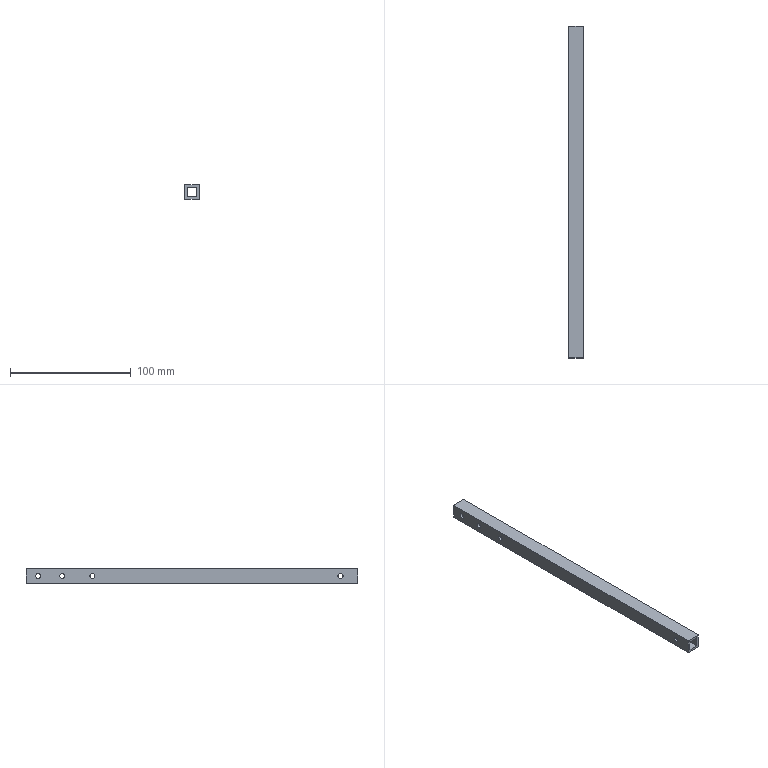Part | SolidWorks | features ICE 3, Extrusion 1 | 1 solid | 26 faces | box 12 x 275 x 12 mm | volume 21786 mm3 | cylinder 16 | plane 10 | commonest cylinder face diameters 4.1 x12 4.2 x4
STEP:
#1=CARTESIAN_POINT('',(6.,265.,-2.05));
#2=VERTEX_POINT('',#1);
#3=CARTESIAN_POINT('',(6.,265.,2.05));
#4=VERTEX_POINT('',#3);
#5=CARTESIAN_POINT('',(6.,265.,0.));
#6=DIRECTION('',(-1.,0.,0.));
#7=DIRECTION('',(0.,0.,1.));
#8=AXIS2_PLACEMENT_3D('',#5,#6,#7);
#9=CIRCLE('',#8,2.05);
#10=EDGE_CURVE('',#2,#4,#9,.T.);
#11=ORIENTED_EDGE('',*,*,#10,.F.);
#12=CARTESIAN_POINT('',(4.,265.,-2.05));
#13=VERTEX_POINT('',#12);
#14=CARTESIAN_POINT('',(6.,265.,-2.05));
#15=DIRECTION('',(-1.,0.,0.));
#16=VECTOR('',#15,1000.);
#17=LINE('',#14,#16);
#18=EDGE_CURVE('',#2,#13,#17,.T.);
#19=ORIENTED_EDGE('',*,*,#18,.T.);
#20=CARTESIAN_POINT('',(4.,265.,2.05));
#21=VERTEX_POINT('',#20);
#22=CARTESIAN_POINT('',(4.,265.,0.));
#23=DIRECTION('',(-1.,0.,0.));
#24=DIRECTION('',(0.,0.,1.));
#25=AXIS2_PLACEMENT_3D('',#22,#23,#24);
#26=CIRCLE('',#25,2.05);
#27=EDGE_CURVE('',#13,#21,#26,.T.);
#28=ORIENTED_EDGE('',*,*,#27,.T.);
#29=CARTESIAN_POINT('',(6.,265.,2.05));
#30=DIRECTION('',(-1.,0.,0.));
#31=VECTOR('',#30,1000.);
#32=LINE('',#29,#31);
#33=EDGE_CURVE('',#4,#21,#32,.T.);
#34=ORIENTED_EDGE('',*,*,#33,.F.);
#35=EDGE_LOOP('',(#11,#19,#28,#34));
#36=FACE_OUTER_BOUND('',#35,.T.);
#37=CARTESIAN_POINT('',(6.,265.,0.));
#38=DIRECTION('',(-1.,0.,0.));
#39=DIRECTION('',(0.,0.,1.));
#40=AXIS2_PLACEMENT_3D('',#37,#38,#39);
#41=CYLINDRICAL_SURFACE('',#40,2.05);
#42=ADVANCED_FACE('',(#36),#41,.F.);
#43=CARTESIAN_POINT('',(6.,245.,-2.05));
#44=VERTEX_POINT('',#43);
#45=CARTESIAN_POINT('',(6.,245.,2.05));
#46=VERTEX_POINT('',#45);
#47=CARTESIAN_POINT('',(6.,245.,0.));
#48=DIRECTION('',(-1.,0.,0.));
#49=DIRECTION('',(0.,0.,1.));
#50=AXIS2_PLACEMENT_3D('',#47,#48,#49);
#51=CIRCLE('',#50,2.05);
#52=EDGE_CURVE('',#44,#46,#51,.T.);
#53=ORIENTED_EDGE('',*,*,#52,.F.);
#54=CARTESIAN_POINT('',(4.,245.,-2.05));
#55=VERTEX_POINT('',#54);
#56=CARTESIAN_POINT('',(6.,245.,-2.05));
#57=DIRECTION('',(-1.,0.,0.));
#58=VECTOR('',#57,1000.);
#59=LINE('',#56,#58);
#60=EDGE_CURVE('',#44,#55,#59,.T.);
#61=ORIENTED_EDGE('',*,*,#60,.T.);
#62=CARTESIAN_POINT('',(4.,245.,2.05));
#63=VERTEX_POINT('',#62);
#64=CARTESIAN_POINT('',(4.,245.,0.));
#65=DIRECTION('',(-1.,0.,0.));
#66=DIRECTION('',(0.,0.,1.));
#67=AXIS2_PLACEMENT_3D('',#64,#65,#66);
#68=CIRCLE('',#67,2.05);
#69=EDGE_CURVE('',#55,#63,#68,.T.);
#70=ORIENTED_EDGE('',*,*,#69,.T.);
#71=CARTESIAN_POINT('',(6.,245.,2.05));
#72=DIRECTION('',(-1.,0.,0.));
#73=VECTOR('',#72,1000.);
#74=LINE('',#71,#73);
#75=EDGE_CURVE('',#46,#63,#74,.T.);
#76=ORIENTED_EDGE('',*,*,#75,.F.);
#77=EDGE_LOOP('',(#53,#61,#70,#76));
#78=FACE_OUTER_BOUND('',#77,.T.);
#79=CARTESIAN_POINT('',(6.,245.,0.));
#80=DIRECTION('',(-1.,0.,0.));
#81=DIRECTION('',(0.,0.,1.));
#82=AXIS2_PLACEMENT_3D('',#79,#80,#81);
#83=CYLINDRICAL_SURFACE('',#82,2.05);
#84=ADVANCED_FACE('',(#78),#83,.F.);
#85=CARTESIAN_POINT('',(6.,220.,-2.05));
#86=VERTEX_POINT('',#85);
#87=CARTESIAN_POINT('',(6.,220.,2.05));
#88=VERTEX_POINT('',#87);
#89=CARTESIAN_POINT('',(6.,220.,0.));
#90=DIRECTION('',(-1.,0.,0.));
#91=DIRECTION('',(0.,0.,1.));
#92=AXIS2_PLACEMENT_3D('',#89,#90,#91);
#93=CIRCLE('',#92,2.05);
#94=EDGE_CURVE('',#86,#88,#93,.T.);
#95=ORIENTED_EDGE('',*,*,#94,.F.);
#96=CARTESIAN_POINT('',(4.,220.,-2.05));
#97=VERTEX_POINT('',#96);
#98=CARTESIAN_POINT('',(6.,220.,-2.05));
#99=DIRECTION('',(-1.,0.,0.));
#100=VECTOR('',#99,1000.);
#101=LINE('',#98,#100);
#102=EDGE_CURVE('',#86,#97,#101,.T.);
#103=ORIENTED_EDGE('',*,*,#102,.T.);
#104=CARTESIAN_POINT('',(4.,220.,2.05));
#105=VERTEX_POINT('',#104);
#106=CARTESIAN_POINT('',(4.,220.,0.));
#107=DIRECTION('',(-1.,0.,0.));
#108=DIRECTION('',(0.,0.,1.));
#109=AXIS2_PLACEMENT_3D('',#106,#107,#108);
#110=CIRCLE('',#109,2.05);
#111=EDGE_CURVE('',#97,#105,#110,.T.);
#112=ORIENTED_EDGE('',*,*,#111,.T.);
#113=CARTESIAN_POINT('',(6.,220.,2.05));
#114=DIRECTION('',(-1.,0.,0.));
#115=VECTOR('',#114,1000.);
#116=LINE('',#113,#115);
#117=EDGE_CURVE('',#88,#105,#116,.T.);
#118=ORIENTED_EDGE('',*,*,#117,.F.);
#119=EDGE_LOOP('',(#95,#103,#112,#118));
#120=FACE_OUTER_BOUND('',#119,.T.);
#121=CARTESIAN_POINT('',(6.,220.,0.));
#122=DIRECTION('',(-1.,0.,0.));
#123=DIRECTION('',(0.,0.,1.));
#124=AXIS2_PLACEMENT_3D('',#121,#122,#123);
#125=CYLINDRICAL_SURFACE('',#124,2.05);
#126=ADVANCED_FACE('',(#120),#125,.F.);
#127=CARTESIAN_POINT('',(6.,14.5,-2.1));
#128=VERTEX_POINT('',#127);
#129=CARTESIAN_POINT('',(6.,14.5,2.1));
#130=VERTEX_POINT('',#129);
#131=CARTESIAN_POINT('',(6.,14.5,0.));
#132=DIRECTION('',(-1.,0.,0.));
#133=DIRECTION('',(0.,0.,1.));
#134=AXIS2_PLACEMENT_3D('',#131,#132,#133);
#135=CIRCLE('',#134,2.1);
#136=EDGE_CURVE('',#128,#130,#135,.T.);
#137=ORIENTED_EDGE('',*,*,#136,.F.);
#138=CARTESIAN_POINT('',(4.,14.5,-2.1));
#139=VERTEX_POINT('',#138);
#140=CARTESIAN_POINT('',(6.,14.5,-2.1));
#141=DIRECTION('',(-1.,0.,0.));
#142=VECTOR('',#141,1000.);
#143=LINE('',#140,#142);
#144=EDGE_CURVE('',#128,#139,#143,.T.);
#145=ORIENTED_EDGE('',*,*,#144,.T.);
#146=CARTESIAN_POINT('',(4.,14.5,2.1));
#147=VERTEX_POINT('',#146);
#148=CARTESIAN_POINT('',(4.,14.5,0.));
#149=DIRECTION('',(-1.,0.,0.));
#150=DIRECTION('',(0.,0.,1.));
#151=AXIS2_PLACEMENT_3D('',#148,#149,#150);
#152=CIRCLE('',#151,2.1);
#153=EDGE_CURVE('',#139,#147,#152,.T.);
#154=ORIENTED_EDGE('',*,*,#153,.T.);
#155=CARTESIAN_POINT('',(6.,14.5,2.1));
#156=DIRECTION('',(-1.,0.,0.));
#157=VECTOR('',#156,1000.);
#158=LINE('',#155,#157);
#159=EDGE_CURVE('',#130,#147,#158,.T.);
#160=ORIENTED_EDGE('',*,*,#159,.F.);
#161=EDGE_LOOP('',(#137,#145,#154,#160));
#162=FACE_OUTER_BOUND('',#161,.T.);
#163=CARTESIAN_POINT('',(6.,14.5,0.));
#164=DIRECTION('',(-1.,0.,0.));
#165=DIRECTION('',(0.,0.,1.));
#166=AXIS2_PLACEMENT_3D('',#163,#164,#165);
#167=CYLINDRICAL_SURFACE('',#166,2.1);
#168=ADVANCED_FACE('',(#162),#167,.F.);
#169=CARTESIAN_POINT('',(-4.,265.,2.05));
#170=VERTEX_POINT('',#169);
#171=CARTESIAN_POINT('',(-4.,265.,-2.05));
#172=VERTEX_POINT('',#171);
#173=CARTESIAN_POINT('',(-4.,265.,0.));
#174=DIRECTION('',(1.,0.,0.));
#175=DIRECTION('',(0.,0.,-1.));
#176=AXIS2_PLACEMENT_3D('',#173,#174,#175);
#177=CIRCLE('',#176,2.05);
#178=EDGE_CURVE('',#170,#172,#177,.T.);
#179=ORIENTED_EDGE('',*,*,#178,.T.);
#180=CARTESIAN_POINT('',(-6.,265.,-2.05));
#181=VERTEX_POINT('',#180);
#182=CARTESIAN_POINT('',(6.,265.,-2.05));
#183=DIRECTION('',(-1.,0.,0.));
#184=VECTOR('',#183,1000.);
#185=LINE('',#182,#184);
#186=EDGE_CURVE('',#172,#181,#185,.T.);
#187=ORIENTED_EDGE('',*,*,#186,.T.);
#188=CARTESIAN_POINT('',(-6.,265.,2.05));
#189=VERTEX_POINT('',#188);
#190=CARTESIAN_POINT('',(-6.,265.,0.));
#191=DIRECTION('',(-1.,0.,0.));
#192=DIRECTION('',(0.,0.,1.));
#193=AXIS2_PLACEMENT_3D('',#190,#191,#192);
#194=CIRCLE('',#193,2.05);
#195=EDGE_CURVE('',#181,#189,#194,.T.);
#196=ORIENTED_EDGE('',*,*,#195,.T.);
#197=CARTESIAN_POINT('',(6.,265.,2.05));
#198=DIRECTION('',(-1.,0.,0.));
#199=VECTOR('',#198,1000.);
#200=LINE('',#197,#199);
#201=EDGE_CURVE('',#170,#189,#200,.T.);
#202=ORIENTED_EDGE('',*,*,#201,.F.);
#203=EDGE_LOOP('',(#179,#187,#196,#202));
#204=FACE_OUTER_BOUND('',#203,.T.);
#205=CARTESIAN_POINT('',(6.,265.,0.));
#206=DIRECTION('',(-1.,0.,0.));
#207=DIRECTION('',(0.,0.,1.));
#208=AXIS2_PLACEMENT_3D('',#205,#206,#207);
#209=CYLINDRICAL_SURFACE('',#208,2.05);
#210=ADVANCED_FACE('',(#204),#209,.F.);
#211=CARTESIAN_POINT('',(-4.,245.,2.05));
#212=VERTEX_POINT('',#211);
#213=CARTESIAN_POINT('',(-4.,245.,-2.05));
#214=VERTEX_POINT('',#213);
#215=CARTESIAN_POINT('',(-4.,245.,0.));
#216=DIRECTION('',(1.,0.,0.));
#217=DIRECTION('',(0.,0.,-1.));
#218=AXIS2_PLACEMENT_3D('',#215,#216,#217);
#219=CIRCLE('',#218,2.05);
#220=EDGE_CURVE('',#212,#214,#219,.T.);
#221=ORIENTED_EDGE('',*,*,#220,.T.);
#222=CARTESIAN_POINT('',(-6.,245.,-2.05));
#223=VERTEX_POINT('',#222);
#224=CARTESIAN_POINT('',(6.,245.,-2.05));
#225=DIRECTION('',(-1.,0.,0.));
#226=VECTOR('',#225,1000.);
#227=LINE('',#224,#226);
#228=EDGE_CURVE('',#214,#223,#227,.T.);
#229=ORIENTED_EDGE('',*,*,#228,.T.);
#230=CARTESIAN_POINT('',(-6.,245.,2.05));
#231=VERTEX_POINT('',#230);
#232=CARTESIAN_POINT('',(-6.,245.,0.));
#233=DIRECTION('',(-1.,0.,0.));
#234=DIRECTION('',(0.,0.,1.));
#235=AXIS2_PLACEMENT_3D('',#232,#233,#234);
#236=CIRCLE('',#235,2.05);
#237=EDGE_CURVE('',#223,#231,#236,.T.);
#238=ORIENTED_EDGE('',*,*,#237,.T.);
#239=CARTESIAN_POINT('',(6.,245.,2.05));
#240=DIRECTION('',(-1.,0.,0.));
#241=VECTOR('',#240,1000.);
#242=LINE('',#239,#241);
#243=EDGE_CURVE('',#212,#231,#242,.T.);
#244=ORIENTED_EDGE('',*,*,#243,.F.);
#245=EDGE_LOOP('',(#221,#229,#238,#244));
#246=FACE_OUTER_BOUND('',#245,.T.);
#247=CARTESIAN_POINT('',(6.,245.,0.));
#248=DIRECTION('',(-1.,0.,0.));
#249=DIRECTION('',(0.,0.,1.));
#250=AXIS2_PLACEMENT_3D('',#247,#248,#249);
#251=CYLINDRICAL_SURFACE('',#250,2.05);
#252=ADVANCED_FACE('',(#246),#251,.F.);
#253=CARTESIAN_POINT('',(-4.,220.,2.05));
#254=VERTEX_POINT('',#253);
#255=CARTESIAN_POINT('',(-4.,220.,-2.05));
#256=VERTEX_POINT('',#255);
#257=CARTESIAN_POINT('',(-4.,220.,0.));
#258=DIRECTION('',(1.,0.,0.));
#259=DIRECTION('',(0.,0.,-1.));
#260=AXIS2_PLACEMENT_3D('',#257,#258,#259);
#261=CIRCLE('',#260,2.05);
#262=EDGE_CURVE('',#254,#256,#261,.T.);
#263=ORIENTED_EDGE('',*,*,#262,.T.);
#264=CARTESIAN_POINT('',(-6.,220.,-2.05));
#265=VERTEX_POINT('',#264);
#266=CARTESIAN_POINT('',(6.,220.,-2.05));
#267=DIRECTION('',(-1.,0.,0.));
#268=VECTOR('',#267,1000.);
#269=LINE('',#266,#268);
#270=EDGE_CURVE('',#256,#265,#269,.T.);
#271=ORIENTED_EDGE('',*,*,#270,.T.);
#272=CARTESIAN_POINT('',(-6.,220.,2.05));
#273=VERTEX_POINT('',#272);
#274=CARTESIAN_POINT('',(-6.,220.,0.));
#275=DIRECTION('',(-1.,0.,0.));
#276=DIRECTION('',(0.,0.,1.));
#277=AXIS2_PLACEMENT_3D('',#274,#275,#276);
#278=CIRCLE('',#277,2.05);
#279=EDGE_CURVE('',#265,#273,#278,.T.);
#280=ORIENTED_EDGE('',*,*,#279,.T.);
#281=CARTESIAN_POINT('',(6.,220.,2.05));
#282=DIRECTION('',(-1.,0.,0.));
#283=VECTOR('',#282,1000.);
#284=LINE('',#281,#283);
#285=EDGE_CURVE('',#254,#273,#284,.T.);
#286=ORIENTED_EDGE('',*,*,#285,.F.);
#287=EDGE_LOOP('',(#263,#271,#280,#286));
#288=FACE_OUTER_BOUND('',#287,.T.);
#289=CARTESIAN_POINT('',(6.,220.,0.));
#290=DIRECTION('',(-1.,0.,0.));
#291=DIRECTION('',(0.,0.,1.));
#292=AXIS2_PLACEMENT_3D('',#289,#290,#291);
#293=CYLINDRICAL_SURFACE('',#292,2.05);
#294=ADVANCED_FACE('',(#288),#293,.F.);
#295=CARTESIAN_POINT('',(-4.,14.5,2.1));
#296=VERTEX_POINT('',#295);
#297=CARTESIAN_POINT('',(-4.,14.5,-2.1));
#298=VERTEX_POINT('',#297);
#299=CARTESIAN_POINT('',(-4.,14.5,0.));
#300=DIRECTION('',(1.,0.,0.));
#301=DIRECTION('',(0.,0.,-1.));
#302=AXIS2_PLACEMENT_3D('',#299,#300,#301);
#303=CIRCLE('',#302,2.1);
#304=EDGE_CURVE('',#296,#298,#303,.T.);
#305=ORIENTED_EDGE('',*,*,#304,.T.);
#306=CARTESIAN_POINT('',(-6.,14.5,-2.1));
#307=VERTEX_POINT('',#306);
#308=CARTESIAN_POINT('',(6.,14.5,-2.1));
#309=DIRECTION('',(-1.,0.,0.));
#310=VECTOR('',#309,1000.);
#311=LINE('',#308,#310);
#312=EDGE_CURVE('',#298,#307,#311,.T.);
#313=ORIENTED_EDGE('',*,*,#312,.T.);
#314=CARTESIAN_POINT('',(-6.,14.5,2.1));
#315=VERTEX_POINT('',#314);
#316=CARTESIAN_POINT('',(-6.,14.5,0.));
#317=DIRECTION('',(-1.,0.,0.));
#318=DIRECTION('',(0.,0.,1.));
#319=AXIS2_PLACEMENT_3D('',#316,#317,#318);
#320=CIRCLE('',#319,2.1);
#321=EDGE_CURVE('',#307,#315,#320,.T.);
#322=ORIENTED_EDGE('',*,*,#321,.T.);
#323=CARTESIAN_POINT('',(6.,14.5,2.1));
#324=DIRECTION('',(-1.,0.,0.));
#325=VECTOR('',#324,1000.);
#326=LINE('',#323,#325);
#327=EDGE_CURVE('',#296,#315,#326,.T.);
#328=ORIENTED_EDGE('',*,*,#327,.F.);
#329=EDGE_LOOP('',(#305,#313,#322,#328));
#330=FACE_OUTER_BOUND('',#329,.T.);
#331=CARTESIAN_POINT('',(6.,14.5,0.));
#332=DIRECTION('',(-1.,0.,0.));
#333=DIRECTION('',(0.,0.,1.));
#334=AXIS2_PLACEMENT_3D('',#331,#332,#333);
#335=CYLINDRICAL_SURFACE('',#334,2.1);
#336=ADVANCED_FACE('',(#330),#335,.F.);
#337=CARTESIAN_POINT('',(6.,275.,6.));
#338=VERTEX_POINT('',#337);
#339=CARTESIAN_POINT('',(6.,275.,-6.));
#340=VERTEX_POINT('',#339);
#341=CARTESIAN_POINT('',(6.,275.,-6.));
#342=DIRECTION('',(0.,0.,-1.));
#343=VECTOR('',#342,1000.);
#344=LINE('',#341,#343);
#345=EDGE_CURVE('',#338,#340,#344,.T.);
#346=ORIENTED_EDGE('',*,*,#345,.T.);
#347=CARTESIAN_POINT('',(-6.,275.,-6.));
#348=VERTEX_POINT('',#347);
#349=CARTESIAN_POINT('',(-6.,275.,-6.));
#350=DIRECTION('',(-1.,0.,0.));
#351=VECTOR('',#350,1000.);
#352=LINE('',#349,#351);
#353=EDGE_CURVE('',#340,#348,#352,.T.);
#354=ORIENTED_EDGE('',*,*,#353,.T.);
#355=CARTESIAN_POINT('',(-6.,275.,6.));
#356=VERTEX_POINT('',#355);
#357=CARTESIAN_POINT('',(-6.,275.,-6.));
#358=DIRECTION('',(0.,0.,1.));
#359=VECTOR('',#358,1000.);
#360=LINE('',#357,#359);
#361=EDGE_CURVE('',#348,#356,#360,.T.);
#362=ORIENTED_EDGE('',*,*,#361,.T.);
#363=CARTESIAN_POINT('',(-6.,275.,6.));
#364=DIRECTION('',(1.,0.,0.));
#365=VECTOR('',#364,1000.);
#366=LINE('',#363,#365);
#367=EDGE_CURVE('',#356,#338,#366,.T.);
#368=ORIENTED_EDGE('',*,*,#367,.T.);
#369=EDGE_LOOP('',(#346,#354,#362,#368));
#370=FACE_OUTER_BOUND('',#369,.T.);
#371=CARTESIAN_POINT('',(4.,275.,-4.));
#372=VERTEX_POINT('',#371);
#373=CARTESIAN_POINT('',(-4.,275.,-4.));
#374=VERTEX_POINT('',#373);
#375=CARTESIAN_POINT('',(-4.,275.,-4.));
#376=DIRECTION('',(-1.,0.,0.));
#377=VECTOR('',#376,1000.);
#378=LINE('',#375,#377);
#379=EDGE_CURVE('',#372,#374,#378,.T.);
#380=ORIENTED_EDGE('',*,*,#379,.F.);
#381=CARTESIAN_POINT('',(4.,275.,4.));
#382=VERTEX_POINT('',#381);
#383=CARTESIAN_POINT('',(4.,275.,-4.));
#384=DIRECTION('',(0.,0.,-1.));
#385=VECTOR('',#384,1000.);
#386=LINE('',#383,#385);
#387=EDGE_CURVE('',#382,#372,#386,.T.);
#388=ORIENTED_EDGE('',*,*,#387,.F.);
#389=CARTESIAN_POINT('',(-4.,275.,4.));
#390=VERTEX_POINT('',#389);
#391=CARTESIAN_POINT('',(-4.,275.,4.));
#392=DIRECTION('',(1.,0.,0.));
#393=VECTOR('',#392,1000.);
#394=LINE('',#391,#393);
#395=EDGE_CURVE('',#390,#382,#394,.T.);
#396=ORIENTED_EDGE('',*,*,#395,.F.);
#397=CARTESIAN_POINT('',(-4.,275.,-4.));
#398=DIRECTION('',(0.,0.,1.));
#399=VECTOR('',#398,1000.);
#400=LINE('',#397,#399);
#401=EDGE_CURVE('',#374,#390,#400,.T.);
#402=ORIENTED_EDGE('',*,*,#401,.F.);
#403=EDGE_LOOP('',(#380,#388,#396,#402));
#404=FACE_BOUND('',#403,.T.);
#405=CARTESIAN_POINT('',(0.,275.,0.));
#406=DIRECTION('',(0.,1.,0.));
#407=DIRECTION('',(0.,0.,1.));
#408=AXIS2_PLACEMENT_3D('',#405,#406,#407);
#409=PLANE('',#408);
#410=ADVANCED_FACE('',(#370,#404),#409,.T.);
#411=CARTESIAN_POINT('',(6.,0.,6.));
#412=VERTEX_POINT('',#411);
#413=CARTESIAN_POINT('',(6.,0.,-6.));
#414=VERTEX_POINT('',#413);
#415=CARTESIAN_POINT('',(6.,0.,-6.));
#416=DIRECTION('',(0.,0.,-1.));
#417=VECTOR('',#416,1000.);
#418=LINE('',#415,#417);
#419=EDGE_CURVE('',#412,#414,#418,.T.);
#420=ORIENTED_EDGE('',*,*,#419,.F.);
#421=CARTESIAN_POINT('',(-6.,0.,6.));
#422=VERTEX_POINT('',#421);
#423=CARTESIAN_POINT('',(-6.,0.,6.));
#424=DIRECTION('',(1.,0.,0.));
#425=VECTOR('',#424,1000.);
#426=LINE('',#423,#425);
#427=EDGE_CURVE('',#422,#412,#426,.T.);
#428=ORIENTED_EDGE('',*,*,#427,.F.);
#429=CARTESIAN_POINT('',(-6.,0.,-6.));
#430=VERTEX_POINT('',#429);
#431=CARTESIAN_POINT('',(-6.,0.,-6.));
#432=DIRECTION('',(0.,0.,1.));
#433=VECTOR('',#432,1000.);
#434=LINE('',#431,#433);
#435=EDGE_CURVE('',#430,#422,#434,.T.);
#436=ORIENTED_EDGE('',*,*,#435,.F.);
#437=CARTESIAN_POINT('',(-6.,0.,-6.));
#438=DIRECTION('',(-1.,0.,0.));
#439=VECTOR('',#438,1000.);
#440=LINE('',#437,#439);
#441=EDGE_CURVE('',#414,#430,#440,.T.);
#442=ORIENTED_EDGE('',*,*,#441,.F.);
#443=EDGE_LOOP('',(#420,#428,#436,#442));
#444=FACE_OUTER_BOUND('',#443,.T.);
#445=CARTESIAN_POINT('',(4.,0.,4.));
#446=VERTEX_POINT('',#445);
#447=CARTESIAN_POINT('',(4.,0.,-4.));
#448=VERTEX_POINT('',#447);
#449=CARTESIAN_POINT('',(4.,0.,-4.));
#450=DIRECTION('',(0.,0.,-1.));
#451=VECTOR('',#450,1000.);
#452=LINE('',#449,#451);
#453=EDGE_CURVE('',#446,#448,#452,.T.);
#454=ORIENTED_EDGE('',*,*,#453,.T.);
#455=CARTESIAN_POINT('',(-4.,0.,-4.));
#456=VERTEX_POINT('',#455);
#457=CARTESIAN_POINT('',(-4.,0.,-4.));
#458=DIRECTION('',(-1.,0.,0.));
#459=VECTOR('',#458,1000.);
#460=LINE('',#457,#459);
#461=EDGE_CURVE('',#448,#456,#460,.T.);
#462=ORIENTED_EDGE('',*,*,#461,.T.);
#463=CARTESIAN_POINT('',(-4.,0.,4.));
#464=VERTEX_POINT('',#463);
#465=CARTESIAN_POINT('',(-4.,0.,-4.));
#466=DIRECTION('',(0.,0.,1.));
#467=VECTOR('',#466,1000.);
#468=LINE('',#465,#467);
#469=EDGE_CURVE('',#456,#464,#468,.T.);
#470=ORIENTED_EDGE('',*,*,#469,.T.);
#471=CARTESIAN_POINT('',(-4.,0.,4.));
#472=DIRECTION('',(1.,0.,0.));
#473=VECTOR('',#472,1000.);
#474=LINE('',#471,#473);
#475=EDGE_CURVE('',#464,#446,#474,.T.);
#476=ORIENTED_EDGE('',*,*,#475,.T.);
#477=EDGE_LOOP('',(#454,#462,#470,#476));
#478=FACE_BOUND('',#477,.T.);
#479=CARTESIAN_POINT('',(0.,0.,0.));
#480=DIRECTION('',(0.,1.,0.));
#481=DIRECTION('',(0.,0.,1.));
#482=AXIS2_PLACEMENT_3D('',#479,#480,#481);
#483=PLANE('',#482);
#484=ADVANCED_FACE('',(#444,#478),#483,.F.);
#485=CARTESIAN_POINT('',(6.,265.,0.));
#486=DIRECTION('',(-1.,0.,0.));
#487=DIRECTION('',(0.,0.,1.));
#488=AXIS2_PLACEMENT_3D('',#485,#486,#487);
#489=CIRCLE('',#488,2.05);
#490=EDGE_CURVE('',#4,#2,#489,.T.);
#491=ORIENTED_EDGE('',*,*,#490,.T.);
#492=ORIENTED_EDGE('',*,*,#10,.T.);
#493=EDGE_LOOP('',(#491,#492));
#494=FACE_BOUND('',#493,.T.);
#495=CARTESIAN_POINT('',(6.,245.,0.));
#496=DIRECTION('',(-1.,0.,0.));
#497=DIRECTION('',(0.,0.,1.));
#498=AXIS2_PLACEMENT_3D('',#495,#496,#497);
#499=CIRCLE('',#498,2.05);
#500=EDGE_CURVE('',#46,#44,#499,.T.);
#501=ORIENTED_EDGE('',*,*,#500,.T.);
#502=ORIENTED_EDGE('',*,*,#52,.T.);
#503=EDGE_LOOP('',(#501,#502));
#504=FACE_BOUND('',#503,.T.);
#505=CARTESIAN_POINT('',(6.,220.,0.));
#506=DIRECTION('',(-1.,0.,0.));
#507=DIRECTION('',(0.,0.,1.));
#508=AXIS2_PLACEMENT_3D('',#505,#506,#507);
#509=CIRCLE('',#508,2.05);
#510=EDGE_CURVE('',#88,#86,#509,.T.);
#511=ORIENTED_EDGE('',*,*,#510,.T.);
#512=ORIENTED_EDGE('',*,*,#94,.T.);
#513=EDGE_LOOP('',(#511,#512));
#514=FACE_BOUND('',#513,.T.);
#515=CARTESIAN_POINT('',(6.,14.5,0.));
#516=DIRECTION('',(-1.,0.,0.));
#517=DIRECTION('',(0.,0.,1.));
#518=AXIS2_PLACEMENT_3D('',#515,#516,#517);
#519=CIRCLE('',#518,2.1);
#520=EDGE_CURVE('',#130,#128,#519,.T.);
#521=ORIENTED_EDGE('',*,*,#520,.T.);
#522=ORIENTED_EDGE('',*,*,#136,.T.);
#523=EDGE_LOOP('',(#521,#522));
#524=FACE_BOUND('',#523,.T.);
#525=ORIENTED_EDGE('',*,*,#419,.T.);
#526=CARTESIAN_POINT('',(6.,275.,-6.));
#527=DIRECTION('',(0.,-1.,0.));
#528=VECTOR('',#527,1000.);
#529=LINE('',#526,#528);
#530=EDGE_CURVE('',#340,#414,#529,.T.);
#531=ORIENTED_EDGE('',*,*,#530,.F.);
#532=ORIENTED_EDGE('',*,*,#345,.F.);
#533=CARTESIAN_POINT('',(6.,275.,6.));
#534=DIRECTION('',(0.,-1.,0.));
#535=VECTOR('',#534,1000.);
#536=LINE('',#533,#535);
#537=EDGE_CURVE('',#338,#412,#536,.T.);
#538=ORIENTED_EDGE('',*,*,#537,.T.);
#539=EDGE_LOOP('',(#525,#531,#532,#538));
#540=FACE_OUTER_BOUND('',#539,.T.);
#541=CARTESIAN_POINT('',(6.,275.,-6.));
#542=DIRECTION('',(-1.,0.,0.));
#543=DIRECTION('',(0.,0.,1.));
#544=AXIS2_PLACEMENT_3D('',#541,#542,#543);
#545=PLANE('',#544);
#546=ADVANCED_FACE('',(#494,#504,#514,#524,#540),#545,.F.);
#547=ORIENTED_EDGE('',*,*,#441,.T.);
#548=CARTESIAN_POINT('',(-6.,275.,-6.));
#549=DIRECTION('',(0.,-1.,0.));
#550=VECTOR('',#549,1000.);
#551=LINE('',#548,#550);
#552=EDGE_CURVE('',#348,#430,#551,.T.);
#553=ORIENTED_EDGE('',*,*,#552,.F.);
#554=ORIENTED_EDGE('',*,*,#353,.F.);
#555=ORIENTED_EDGE('',*,*,#530,.T.);
#556=EDGE_LOOP('',(#547,#553,#554,#555));
#557=FACE_OUTER_BOUND('',#556,.T.);
#558=CARTESIAN_POINT('',(-6.,275.,-6.));
#559=DIRECTION('',(0.,0.,1.));
#560=DIRECTION('',(1.,0.,0.));
#561=AXIS2_PLACEMENT_3D('',#558,#559,#560);
#562=PLANE('',#561);
#563=ADVANCED_FACE('',(#557),#562,.F.);
#564=CARTESIAN_POINT('',(-6.,265.,0.));
#565=DIRECTION('',(-1.,0.,0.));
#566=DIRECTION('',(0.,0.,1.));
#567=AXIS2_PLACEMENT_3D('',#564,#565,#566);
#568=CIRCLE('',#567,2.05);
#569=EDGE_CURVE('',#189,#181,#568,.T.);
#570=ORIENTED_EDGE('',*,*,#569,.F.);
#571=ORIENTED_EDGE('',*,*,#195,.F.);
#572=EDGE_LOOP('',(#570,#571));
#573=FACE_BOUND('',#572,.T.);
#574=CARTESIAN_POINT('',(-6.,245.,0.));
#575=DIRECTION('',(-1.,0.,0.));
#576=DIRECTION('',(0.,0.,1.));
#577=AXIS2_PLACEMENT_3D('',#574,#575,#576);
#578=CIRCLE('',#577,2.05);
#579=EDGE_CURVE('',#231,#223,#578,.T.);
#580=ORIENTED_EDGE('',*,*,#579,.F.);
#581=ORIENTED_EDGE('',*,*,#237,.F.);
#582=EDGE_LOOP('',(#580,#581));
#583=FACE_BOUND('',#582,.T.);
#584=CARTESIAN_POINT('',(-6.,220.,0.));
#585=DIRECTION('',(-1.,0.,0.));
#586=DIRECTION('',(0.,0.,1.));
#587=AXIS2_PLACEMENT_3D('',#584,#585,#586);
#588=CIRCLE('',#587,2.05);
#589=EDGE_CURVE('',#273,#265,#588,.T.);
#590=ORIENTED_EDGE('',*,*,#589,.F.);
#591=ORIENTED_EDGE('',*,*,#279,.F.);
#592=EDGE_LOOP('',(#590,#591));
#593=FACE_BOUND('',#592,.T.);
#594=CARTESIAN_POINT('',(-6.,14.5,0.));
#595=DIRECTION('',(-1.,0.,0.));
#596=DIRECTION('',(0.,0.,1.));
#597=AXIS2_PLACEMENT_3D('',#594,#595,#596);
#598=CIRCLE('',#597,2.1);
#599=EDGE_CURVE('',#315,#307,#598,.T.);
#600=ORIENTED_EDGE('',*,*,#599,.F.);
#601=ORIENTED_EDGE('',*,*,#321,.F.);
#602=EDGE_LOOP('',(#600,#601));
#603=FACE_BOUND('',#602,.T.);
#604=ORIENTED_EDGE('',*,*,#435,.T.);
#605=CARTESIAN_POINT('',(-6.,275.,6.));
#606=DIRECTION('',(0.,-1.,0.));
#607=VECTOR('',#606,1000.);
#608=LINE('',#605,#607);
#609=EDGE_CURVE('',#356,#422,#608,.T.);
#610=ORIENTED_EDGE('',*,*,#609,.F.);
#611=ORIENTED_EDGE('',*,*,#361,.F.);
#612=ORIENTED_EDGE('',*,*,#552,.T.);
#613=EDGE_LOOP('',(#604,#610,#611,#612));
#614=FACE_OUTER_BOUND('',#613,.T.);
#615=CARTESIAN_POINT('',(-6.,275.,-6.));
#616=DIRECTION('',(1.,0.,0.));
#617=DIRECTION('',(0.,0.,-1.));
#618=AXIS2_PLACEMENT_3D('',#615,#616,#617);
#619=PLANE('',#618);
#620=ADVANCED_FACE('',(#573,#583,#593,#603,#614),#619,.F.);
#621=ORIENTED_EDGE('',*,*,#427,.T.);
#622=ORIENTED_EDGE('',*,*,#537,.F.);
#623=ORIENTED_EDGE('',*,*,#367,.F.);
#624=ORIENTED_EDGE('',*,*,#609,.T.);
#625=EDGE_LOOP('',(#621,#622,#623,#624));
#626=FACE_OUTER_BOUND('',#625,.T.);
#627=CARTESIAN_POINT('',(-6.,275.,6.));
#628=DIRECTION('',(0.,0.,-1.));
#629=DIRECTION('',(-1.,0.,0.));
#630=AXIS2_PLACEMENT_3D('',#627,#628,#629);
#631=PLANE('',#630);
#632=ADVANCED_FACE('',(#626),#631,.F.);
#633=CARTESIAN_POINT('',(4.,265.,0.));
#634=DIRECTION('',(-1.,0.,0.));
#635=DIRECTION('',(0.,0.,1.));
#636=AXIS2_PLACEMENT_3D('',#633,#634,#635);
#637=CIRCLE('',#636,2.05);
#638=EDGE_CURVE('',#21,#13,#637,.T.);
#639=ORIENTED_EDGE('',*,*,#638,.F.);
#640=ORIENTED_EDGE('',*,*,#27,.F.);
#641=EDGE_LOOP('',(#639,#640));
#642=FACE_BOUND('',#641,.T.);
#643=CARTESIAN_POINT('',(4.,245.,0.));
#644=DIRECTION('',(-1.,0.,0.));
#645=DIRECTION('',(0.,0.,1.));
#646=AXIS2_PLACEMENT_3D('',#643,#644,#645);
#647=CIRCLE('',#646,2.05);
#648=EDGE_CURVE('',#63,#55,#647,.T.);
#649=ORIENTED_EDGE('',*,*,#648,.F.);
#650=ORIENTED_EDGE('',*,*,#69,.F.);
#651=EDGE_LOOP('',(#649,#650));
#652=FACE_BOUND('',#651,.T.);
#653=CARTESIAN_POINT('',(4.,220.,0.));
#654=DIRECTION('',(-1.,0.,0.));
#655=DIRECTION('',(0.,0.,1.));
#656=AXIS2_PLACEMENT_3D('',#653,#654,#655);
#657=CIRCLE('',#656,2.05);
#658=EDGE_CURVE('',#105,#97,#657,.T.);
#659=ORIENTED_EDGE('',*,*,#658,.F.);
#660=ORIENTED_EDGE('',*,*,#111,.F.);
#661=EDGE_LOOP('',(#659,#660));
#662=FACE_BOUND('',#661,.T.);
#663=CARTESIAN_POINT('',(4.,14.5,0.));
#664=DIRECTION('',(-1.,0.,0.));
#665=DIRECTION('',(0.,0.,1.));
#666=AXIS2_PLACEMENT_3D('',#663,#664,#665);
#667=CIRCLE('',#666,2.1);
#668=EDGE_CURVE('',#147,#139,#667,.T.);
#669=ORIENTED_EDGE('',*,*,#668,.F.);
#670=ORIENTED_EDGE('',*,*,#153,.F.);
#671=EDGE_LOOP('',(#669,#670));
#672=FACE_BOUND('',#671,.T.);
#673=ORIENTED_EDGE('',*,*,#453,.F.);
#674=CARTESIAN_POINT('',(4.,275.,4.));
#675=DIRECTION('',(0.,-1.,0.));
#676=VECTOR('',#675,1000.);
#677=LINE('',#674,#676);
#678=EDGE_CURVE('',#382,#446,#677,.T.);
#679=ORIENTED_EDGE('',*,*,#678,.F.);
#680=ORIENTED_EDGE('',*,*,#387,.T.);
#681=CARTESIAN_POINT('',(4.,275.,-4.));
#682=DIRECTION('',(0.,-1.,0.));
#683=VECTOR('',#682,1000.);
#684=LINE('',#681,#683);
#685=EDGE_CURVE('',#372,#448,#684,.T.);
#686=ORIENTED_EDGE('',*,*,#685,.T.);
#687=EDGE_LOOP('',(#673,#679,#680,#686));
#688=FACE_OUTER_BOUND('',#687,.T.);
#689=CARTESIAN_POINT('',(4.,275.,-4.));
#690=DIRECTION('',(-1.,0.,0.));
#691=DIRECTION('',(0.,0.,1.));
#692=AXIS2_PLACEMENT_3D('',#689,#690,#691);
#693=PLANE('',#692);
#694=ADVANCED_FACE('',(#642,#652,#662,#672,#688),#693,.T.);
#695=ORIENTED_EDGE('',*,*,#461,.F.);
#696=ORIENTED_EDGE('',*,*,#685,.F.);
#697=ORIENTED_EDGE('',*,*,#379,.T.);
#698=CARTESIAN_POINT('',(-4.,275.,-4.));
#699=DIRECTION('',(0.,-1.,0.));
#700=VECTOR('',#699,1000.);
#701=LINE('',#698,#700);
#702=EDGE_CURVE('',#374,#456,#701,.T.);
#703=ORIENTED_EDGE('',*,*,#702,.T.);
#704=EDGE_LOOP('',(#695,#696,#697,#703));
#705=FACE_OUTER_BOUND('',#704,.T.);
#706=CARTESIAN_POINT('',(-4.,275.,-4.));
#707=DIRECTION('',(0.,0.,1.));
#708=DIRECTION('',(1.,0.,0.));
#709=AXIS2_PLACEMENT_3D('',#706,#707,#708);
#710=PLANE('',#709);
#711=ADVANCED_FACE('',(#705),#710,.T.);
#712=ORIENTED_EDGE('',*,*,#178,.F.);
#713=CARTESIAN_POINT('',(-4.,265.,0.));
#714=DIRECTION('',(1.,0.,0.));
#715=DIRECTION('',(0.,0.,-1.));
#716=AXIS2_PLACEMENT_3D('',#713,#714,#715);
#717=CIRCLE('',#716,2.05);
#718=EDGE_CURVE('',#172,#170,#717,.T.);
#719=ORIENTED_EDGE('',*,*,#718,.F.);
#720=EDGE_LOOP('',(#712,#719));
#721=FACE_BOUND('',#720,.T.);
#722=ORIENTED_EDGE('',*,*,#220,.F.);
#723=CARTESIAN_POINT('',(-4.,245.,0.));
#724=DIRECTION('',(1.,0.,0.));
#725=DIRECTION('',(0.,0.,-1.));
#726=AXIS2_PLACEMENT_3D('',#723,#724,#725);
#727=CIRCLE('',#726,2.05);
#728=EDGE_CURVE('',#214,#212,#727,.T.);
#729=ORIENTED_EDGE('',*,*,#728,.F.);
#730=EDGE_LOOP('',(#722,#729));
#731=FACE_BOUND('',#730,.T.);
#732=ORIENTED_EDGE('',*,*,#262,.F.);
#733=CARTESIAN_POINT('',(-4.,220.,0.));
#734=DIRECTION('',(1.,0.,0.));
#735=DIRECTION('',(0.,0.,-1.));
#736=AXIS2_PLACEMENT_3D('',#733,#734,#735);
#737=CIRCLE('',#736,2.05);
#738=EDGE_CURVE('',#256,#254,#737,.T.);
#739=ORIENTED_EDGE('',*,*,#738,.F.);
#740=EDGE_LOOP('',(#732,#739));
#741=FACE_BOUND('',#740,.T.);
#742=ORIENTED_EDGE('',*,*,#304,.F.);
#743=CARTESIAN_POINT('',(-4.,14.5,0.));
#744=DIRECTION('',(1.,0.,0.));
#745=DIRECTION('',(0.,0.,-1.));
#746=AXIS2_PLACEMENT_3D('',#743,#744,#745);
#747=CIRCLE('',#746,2.1);
#748=EDGE_CURVE('',#298,#296,#747,.T.);
#749=ORIENTED_EDGE('',*,*,#748,.F.);
#750=EDGE_LOOP('',(#742,#749));
#751=FACE_BOUND('',#750,.T.);
#752=ORIENTED_EDGE('',*,*,#469,.F.);
#753=ORIENTED_EDGE('',*,*,#702,.F.);
#754=ORIENTED_EDGE('',*,*,#401,.T.);
#755=CARTESIAN_POINT('',(-4.,275.,4.));
#756=DIRECTION('',(0.,-1.,0.));
#757=VECTOR('',#756,1000.);
#758=LINE('',#755,#757);
#759=EDGE_CURVE('',#390,#464,#758,.T.);
#760=ORIENTED_EDGE('',*,*,#759,.T.);
#761=EDGE_LOOP('',(#752,#753,#754,#760));
#762=FACE_OUTER_BOUND('',#761,.T.);
#763=CARTESIAN_POINT('',(-4.,275.,-4.));
#764=DIRECTION('',(1.,0.,0.));
#765=DIRECTION('',(0.,0.,-1.));
#766=AXIS2_PLACEMENT_3D('',#763,#764,#765);
#767=PLANE('',#766);
#768=ADVANCED_FACE('',(#721,#731,#741,#751,#762),#767,.T.);
#769=ORIENTED_EDGE('',*,*,#475,.F.);
#770=ORIENTED_EDGE('',*,*,#759,.F.);
#771=ORIENTED_EDGE('',*,*,#395,.T.);
#772=ORIENTED_EDGE('',*,*,#678,.T.);
#773=EDGE_LOOP('',(#769,#770,#771,#772));
#774=FACE_OUTER_BOUND('',#773,.T.);
#775=CARTESIAN_POINT('',(-4.,275.,4.));
#776=DIRECTION('',(0.,0.,-1.));
#777=DIRECTION('',(-1.,0.,0.));
#778=AXIS2_PLACEMENT_3D('',#775,#776,#777);
#779=PLANE('',#778);
#780=ADVANCED_FACE('',(#774),#779,.T.);
#781=ORIENTED_EDGE('',*,*,#312,.F.);
#782=ORIENTED_EDGE('',*,*,#748,.T.);
#783=ORIENTED_EDGE('',*,*,#327,.T.);
#784=ORIENTED_EDGE('',*,*,#599,.T.);
#785=EDGE_LOOP('',(#781,#782,#783,#784));
#786=FACE_OUTER_BOUND('',#785,.T.);
#787=CARTESIAN_POINT('',(6.,14.5,0.));
#788=DIRECTION('',(-1.,0.,0.));
#789=DIRECTION('',(0.,0.,1.));
#790=AXIS2_PLACEMENT_3D('',#787,#788,#789);
#791=CYLINDRICAL_SURFACE('',#790,2.1);
#792=ADVANCED_FACE('',(#786),#791,.F.);
#793=ORIENTED_EDGE('',*,*,#270,.F.);
#794=ORIENTED_EDGE('',*,*,#738,.T.);
#795=ORIENTED_EDGE('',*,*,#285,.T.);
#796=ORIENTED_EDGE('',*,*,#589,.T.);
#797=EDGE_LOOP('',(#793,#794,#795,#796));
#798=FACE_OUTER_BOUND('',#797,.T.);
#799=CARTESIAN_POINT('',(6.,220.,0.));
#800=DIRECTION('',(-1.,0.,0.));
#801=DIRECTION('',(0.,0.,1.));
#802=AXIS2_PLACEMENT_3D('',#799,#800,#801);
#803=CYLINDRICAL_SURFACE('',#802,2.05);
#804=ADVANCED_FACE('',(#798),#803,.F.);
#805=ORIENTED_EDGE('',*,*,#228,.F.);
#806=ORIENTED_EDGE('',*,*,#728,.T.);
#807=ORIENTED_EDGE('',*,*,#243,.T.);
#808=ORIENTED_EDGE('',*,*,#579,.T.);
#809=EDGE_LOOP('',(#805,#806,#807,#808));
#810=FACE_OUTER_BOUND('',#809,.T.);
#811=CARTESIAN_POINT('',(6.,245.,0.));
#812=DIRECTION('',(-1.,0.,0.));
#813=DIRECTION('',(0.,0.,1.));
#814=AXIS2_PLACEMENT_3D('',#811,#812,#813);
#815=CYLINDRICAL_SURFACE('',#814,2.05);
#816=ADVANCED_FACE('',(#810),#815,.F.);
#817=ORIENTED_EDGE('',*,*,#186,.F.);
#818=ORIENTED_EDGE('',*,*,#718,.T.);
#819=ORIENTED_EDGE('',*,*,#201,.T.);
#820=ORIENTED_EDGE('',*,*,#569,.T.);
#821=EDGE_LOOP('',(#817,#818,#819,#820));
#822=FACE_OUTER_BOUND('',#821,.T.);
#823=CARTESIAN_POINT('',(6.,265.,0.));
#824=DIRECTION('',(-1.,0.,0.));
#825=DIRECTION('',(0.,0.,1.));
#826=AXIS2_PLACEMENT_3D('',#823,#824,#825);
#827=CYLINDRICAL_SURFACE('',#826,2.05);
#828=ADVANCED_FACE('',(#822),#827,.F.);
#829=ORIENTED_EDGE('',*,*,#144,.F.);
#830=ORIENTED_EDGE('',*,*,#520,.F.);
#831=ORIENTED_EDGE('',*,*,#159,.T.);
#832=ORIENTED_EDGE('',*,*,#668,.T.);
#833=EDGE_LOOP('',(#829,#830,#831,#832));
#834=FACE_OUTER_BOUND('',#833,.T.);
#835=CARTESIAN_POINT('',(6.,14.5,0.));
#836=DIRECTION('',(-1.,0.,0.));
#837=DIRECTION('',(0.,0.,1.));
#838=AXIS2_PLACEMENT_3D('',#835,#836,#837);
#839=CYLINDRICAL_SURFACE('',#838,2.1);
#840=ADVANCED_FACE('',(#834),#839,.F.);
#841=ORIENTED_EDGE('',*,*,#102,.F.);
#842=ORIENTED_EDGE('',*,*,#510,.F.);
#843=ORIENTED_EDGE('',*,*,#117,.T.);
#844=ORIENTED_EDGE('',*,*,#658,.T.);
#845=EDGE_LOOP('',(#841,#842,#843,#844));
#846=FACE_OUTER_BOUND('',#845,.T.);
#847=CARTESIAN_POINT('',(6.,220.,0.));
#848=DIRECTION('',(-1.,0.,0.));
#849=DIRECTION('',(0.,0.,1.));
#850=AXIS2_PLACEMENT_3D('',#847,#848,#849);
#851=CYLINDRICAL_SURFACE('',#850,2.05);
#852=ADVANCED_FACE('',(#846),#851,.F.);
#853=ORIENTED_EDGE('',*,*,#60,.F.);
#854=ORIENTED_EDGE('',*,*,#500,.F.);
#855=ORIENTED_EDGE('',*,*,#75,.T.);
#856=ORIENTED_EDGE('',*,*,#648,.T.);
#857=EDGE_LOOP('',(#853,#854,#855,#856));
#858=FACE_OUTER_BOUND('',#857,.T.);
#859=CARTESIAN_POINT('',(6.,245.,0.));
#860=DIRECTION('',(-1.,0.,0.));
#861=DIRECTION('',(0.,0.,1.));
#862=AXIS2_PLACEMENT_3D('',#859,#860,#861);
#863=CYLINDRICAL_SURFACE('',#862,2.05);
#864=ADVANCED_FACE('',(#858),#863,.F.);
#865=ORIENTED_EDGE('',*,*,#18,.F.);
#866=ORIENTED_EDGE('',*,*,#490,.F.);
#867=ORIENTED_EDGE('',*,*,#33,.T.);
#868=ORIENTED_EDGE('',*,*,#638,.T.);
#869=EDGE_LOOP('',(#865,#866,#867,#868));
#870=FACE_OUTER_BOUND('',#869,.T.);
#871=CARTESIAN_POINT('',(6.,265.,0.));
#872=DIRECTION('',(-1.,0.,0.));
#873=DIRECTION('',(0.,0.,1.));
#874=AXIS2_PLACEMENT_3D('',#871,#872,#873);
#875=CYLINDRICAL_SURFACE('',#874,2.05);
#876=ADVANCED_FACE('',(#870),#875,.F.);
#877=CLOSED_SHELL('',(#42,#84,#126,#168,#210,#252,#294,#336,#410,#484,#546,#563,#620,#632,#694,#711,#768,#780,#792,#804,#816,#828,#840,#852,#864,#876));
#878=MANIFOLD_SOLID_BREP('',#877);
#879=CARTESIAN_POINT('',(0.,0.,0.));
#880=DIRECTION('',(0.,0.,1.));
#881=DIRECTION('',(1.,0.,0.));
#882=AXIS2_PLACEMENT_3D('',#879,#880,#881);
#883=(LENGTH_UNIT()NAMED_UNIT(*)SI_UNIT(.MILLI.,.METRE.));
#884=UNCERTAINTY_MEASURE_WITH_UNIT(LENGTH_MEASURE(0.00001),#883,'','');
#885=(NAMED_UNIT(*)PLANE_ANGLE_UNIT()SI_UNIT($,.RADIAN.));
#886=(NAMED_UNIT(*)SI_UNIT($,.STERADIAN.)SOLID_ANGLE_UNIT());
#887=(GEOMETRIC_REPRESENTATION_CONTEXT(3)GLOBAL_UNCERTAINTY_ASSIGNED_CONTEXT((#884))GLOBAL_UNIT_ASSIGNED_CONTEXT((#883,#885,#886))REPRESENTATION_CONTEXT('',''));
#888=ADVANCED_BREP_SHAPE_REPRESENTATION('',(#878,#882),#887);